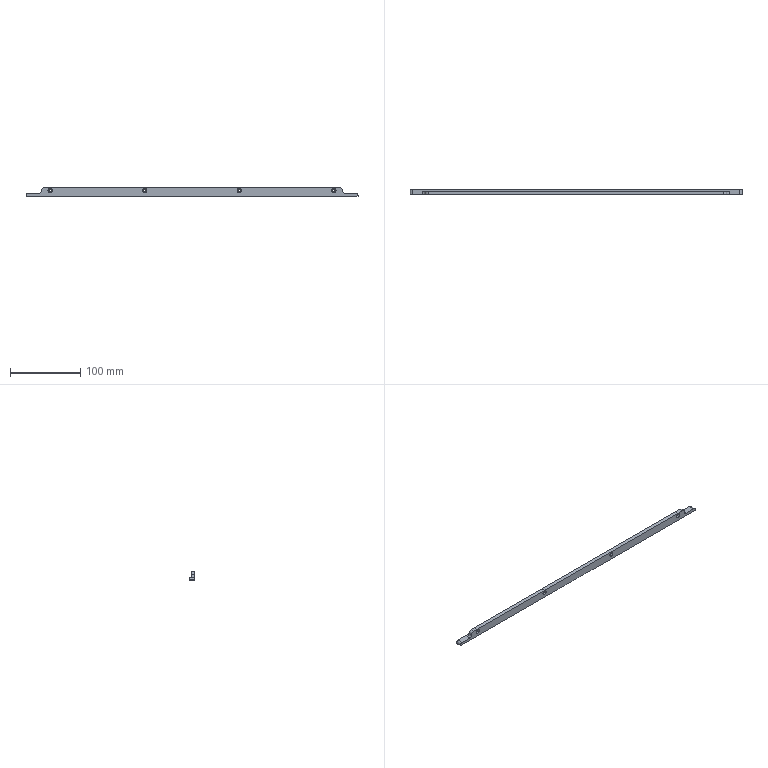Part | NX | 1 solid | 28 faces | box 474 x 8.3 x 12 mm | volume 32389 mm3 | cylinder 14 | plane 14 | commonest cylinder face diameters 3.4 x4 6.5 x4 8 x4 6 x2
STEP:
#1=CARTESIAN_POINT('',(22.,0.,-4.));
#2=VERTEX_POINT('',#1);
#3=CARTESIAN_POINT('',(18.,0.,-8.));
#4=VERTEX_POINT('',#3);
#5=CARTESIAN_POINT('',(18.,0.,-4.));
#6=DIRECTION('',(0.,1.,0.));
#7=DIRECTION('',(0.,0.,-1.));
#8=AXIS2_PLACEMENT_3D('',#5,#6,#7);
#9=CIRCLE('',#8,4.);
#10=EDGE_CURVE('',#2,#4,#9,.T.);
#11=ORIENTED_EDGE('',*,*,#10,.F.);
#12=CARTESIAN_POINT('',(22.,5.,-4.));
#13=VERTEX_POINT('',#12);
#14=CARTESIAN_POINT('',(22.,0.,-4.));
#15=DIRECTION('',(0.,1.,0.));
#16=VECTOR('',#15,1000.);
#17=LINE('',#14,#16);
#18=EDGE_CURVE('',#2,#13,#17,.T.);
#19=ORIENTED_EDGE('',*,*,#18,.T.);
#20=CARTESIAN_POINT('',(18.,5.,-8.));
#21=VERTEX_POINT('',#20);
#22=CARTESIAN_POINT('',(18.,5.,-4.));
#23=DIRECTION('',(0.,-1.,0.));
#24=DIRECTION('',(0.,0.,-1.));
#25=AXIS2_PLACEMENT_3D('',#22,#23,#24);
#26=CIRCLE('',#25,4.);
#27=EDGE_CURVE('',#21,#13,#26,.T.);
#28=ORIENTED_EDGE('',*,*,#27,.F.);
#29=CARTESIAN_POINT('',(18.,8.3,-8.));
#30=DIRECTION('',(0.,1.,0.));
#31=VECTOR('',#30,1000.);
#32=LINE('',#29,#31);
#33=EDGE_CURVE('',#4,#21,#32,.T.);
#34=ORIENTED_EDGE('',*,*,#33,.F.);
#35=EDGE_LOOP('',(#11,#19,#28,#34));
#36=FACE_BOUND('',#35,.T.);
#37=CARTESIAN_POINT('',(18.,-5.,-4.));
#38=DIRECTION('',(0.,1.,0.));
#39=DIRECTION('',(0.,0.,1.));
#40=AXIS2_PLACEMENT_3D('',#37,#38,#39);
#41=CYLINDRICAL_SURFACE('',#40,4.);
#42=ADVANCED_FACE('',(#36),#41,.F.);
#43=ORIENTED_EDGE('',*,*,#18,.F.);
#44=CARTESIAN_POINT('',(26.,0.,0.));
#45=VERTEX_POINT('',#44);
#46=CARTESIAN_POINT('',(26.,0.,-4.));
#47=DIRECTION('',(0.,-1.,0.));
#48=DIRECTION('',(0.,0.,-1.));
#49=AXIS2_PLACEMENT_3D('',#46,#47,#48);
#50=CIRCLE('',#49,4.);
#51=EDGE_CURVE('',#45,#2,#50,.T.);
#52=ORIENTED_EDGE('',*,*,#51,.F.);
#53=CARTESIAN_POINT('',(26.,5.,0.));
#54=VERTEX_POINT('',#53);
#55=CARTESIAN_POINT('',(26.,5.,0.));
#56=DIRECTION('',(0.,1.,0.));
#57=VECTOR('',#56,1000.);
#58=LINE('',#55,#57);
#59=EDGE_CURVE('',#54,#45,#58,.F.);
#60=ORIENTED_EDGE('',*,*,#59,.F.);
#61=CARTESIAN_POINT('',(26.,5.,-4.));
#62=DIRECTION('',(0.,1.,0.));
#63=DIRECTION('',(0.,0.,-1.));
#64=AXIS2_PLACEMENT_3D('',#61,#62,#63);
#65=CIRCLE('',#64,4.);
#66=EDGE_CURVE('',#13,#54,#65,.T.);
#67=ORIENTED_EDGE('',*,*,#66,.F.);
#68=EDGE_LOOP('',(#43,#52,#60,#67));
#69=FACE_BOUND('',#68,.T.);
#70=CARTESIAN_POINT('',(26.,-5.,-4.));
#71=DIRECTION('',(0.,1.,0.));
#72=DIRECTION('',(0.,0.,1.));
#73=AXIS2_PLACEMENT_3D('',#70,#71,#72);
#74=CYLINDRICAL_SURFACE('',#73,4.);
#75=ADVANCED_FACE('',(#69),#74,.T.);
#76=CARTESIAN_POINT('',(452.,0.,-4.));
#77=VERTEX_POINT('',#76);
#78=CARTESIAN_POINT('',(448.,0.,0.));
#79=VERTEX_POINT('',#78);
#80=CARTESIAN_POINT('',(448.,0.,-4.));
#81=DIRECTION('',(0.,-1.,0.));
#82=DIRECTION('',(0.,0.,-1.));
#83=AXIS2_PLACEMENT_3D('',#80,#81,#82);
#84=CIRCLE('',#83,4.);
#85=EDGE_CURVE('',#77,#79,#84,.T.);
#86=ORIENTED_EDGE('',*,*,#85,.F.);
#87=CARTESIAN_POINT('',(452.,5.,-4.));
#88=VERTEX_POINT('',#87);
#89=CARTESIAN_POINT('',(452.,0.,-4.));
#90=DIRECTION('',(0.,-1.,0.));
#91=VECTOR('',#90,1000.);
#92=LINE('',#89,#91);
#93=EDGE_CURVE('',#77,#88,#92,.F.);
#94=ORIENTED_EDGE('',*,*,#93,.T.);
#95=CARTESIAN_POINT('',(448.,5.,0.));
#96=VERTEX_POINT('',#95);
#97=CARTESIAN_POINT('',(448.,5.,-4.));
#98=DIRECTION('',(0.,1.,0.));
#99=DIRECTION('',(0.,0.,-1.));
#100=AXIS2_PLACEMENT_3D('',#97,#98,#99);
#101=CIRCLE('',#100,4.);
#102=EDGE_CURVE('',#96,#88,#101,.T.);
#103=ORIENTED_EDGE('',*,*,#102,.F.);
#104=CARTESIAN_POINT('',(448.,5.,0.));
#105=DIRECTION('',(0.,-1.,0.));
#106=VECTOR('',#105,1000.);
#107=LINE('',#104,#106);
#108=EDGE_CURVE('',#79,#96,#107,.F.);
#109=ORIENTED_EDGE('',*,*,#108,.F.);
#110=EDGE_LOOP('',(#86,#94,#103,#109));
#111=FACE_BOUND('',#110,.T.);
#112=CARTESIAN_POINT('',(448.,-5.,-4.));
#113=DIRECTION('',(0.,-1.,0.));
#114=DIRECTION('',(0.,0.,-1.));
#115=AXIS2_PLACEMENT_3D('',#112,#113,#114);
#116=CYLINDRICAL_SURFACE('',#115,4.);
#117=ADVANCED_FACE('',(#111),#116,.T.);
#118=ORIENTED_EDGE('',*,*,#93,.F.);
#119=CARTESIAN_POINT('',(456.,0.,-8.));
#120=VERTEX_POINT('',#119);
#121=CARTESIAN_POINT('',(456.,0.,-4.));
#122=DIRECTION('',(0.,1.,0.));
#123=DIRECTION('',(0.,0.,-1.));
#124=AXIS2_PLACEMENT_3D('',#121,#122,#123);
#125=CIRCLE('',#124,4.);
#126=EDGE_CURVE('',#120,#77,#125,.T.);
#127=ORIENTED_EDGE('',*,*,#126,.F.);
#128=CARTESIAN_POINT('',(456.,5.,-8.));
#129=VERTEX_POINT('',#128);
#130=CARTESIAN_POINT('',(456.,8.3,-8.));
#131=DIRECTION('',(0.,-1.,0.));
#132=VECTOR('',#131,1000.);
#133=LINE('',#130,#132);
#134=EDGE_CURVE('',#129,#120,#133,.T.);
#135=ORIENTED_EDGE('',*,*,#134,.F.);
#136=CARTESIAN_POINT('',(456.,5.,-4.));
#137=DIRECTION('',(0.,-1.,0.));
#138=DIRECTION('',(0.,0.,-1.));
#139=AXIS2_PLACEMENT_3D('',#136,#137,#138);
#140=CIRCLE('',#139,4.);
#141=EDGE_CURVE('',#88,#129,#140,.T.);
#142=ORIENTED_EDGE('',*,*,#141,.F.);
#143=EDGE_LOOP('',(#118,#127,#135,#142));
#144=FACE_BOUND('',#143,.T.);
#145=CARTESIAN_POINT('',(456.,-5.,-4.));
#146=DIRECTION('',(0.,-1.,0.));
#147=DIRECTION('',(0.,0.,-1.));
#148=AXIS2_PLACEMENT_3D('',#145,#146,#147);
#149=CYLINDRICAL_SURFACE('',#148,4.);
#150=ADVANCED_FACE('',(#144),#149,.F.);
#151=CARTESIAN_POINT('',(34.5,3.4,-7.25));
#152=VERTEX_POINT('',#151);
#153=CARTESIAN_POINT('',(34.5,3.4,-4.));
#154=DIRECTION('',(0.,-1.,0.));
#155=DIRECTION('',(0.,0.,-1.));
#156=AXIS2_PLACEMENT_3D('',#153,#154,#155);
#157=CIRCLE('',#156,3.25);
#158=EDGE_CURVE('',#152,#152,#157,.T.);
#159=ORIENTED_EDGE('',*,*,#158,.T.);
#160=EDGE_LOOP('',(#159));
#161=FACE_BOUND('',#160,.T.);
#162=CARTESIAN_POINT('',(34.5,3.4,-5.7));
#163=VERTEX_POINT('',#162);
#164=CARTESIAN_POINT('',(34.5,3.4,-4.));
#165=DIRECTION('',(0.,-1.,0.));
#166=DIRECTION('',(0.,0.,-1.));
#167=AXIS2_PLACEMENT_3D('',#164,#165,#166);
#168=CIRCLE('',#167,1.7);
#169=EDGE_CURVE('',#163,#163,#168,.T.);
#170=ORIENTED_EDGE('',*,*,#169,.F.);
#171=EDGE_LOOP('',(#170));
#172=FACE_BOUND('',#171,.T.);
#173=CARTESIAN_POINT('',(36.2,3.4,-4.));
#174=DIRECTION('',(0.,1.,0.));
#175=DIRECTION('',(0.,0.,1.));
#176=AXIS2_PLACEMENT_3D('',#173,#174,#175);
#177=PLANE('',#176);
#178=ADVANCED_FACE('',(#161,#172),#177,.F.);
#179=CARTESIAN_POINT('',(169.5,3.4,-0.75));
#180=VERTEX_POINT('',#179);
#181=CARTESIAN_POINT('',(169.5,3.4,-4.));
#182=DIRECTION('',(0.,-1.,0.));
#183=DIRECTION('',(0.,0.,1.));
#184=AXIS2_PLACEMENT_3D('',#181,#182,#183);
#185=CIRCLE('',#184,3.25);
#186=EDGE_CURVE('',#180,#180,#185,.T.);
#187=ORIENTED_EDGE('',*,*,#186,.T.);
#188=EDGE_LOOP('',(#187));
#189=FACE_BOUND('',#188,.T.);
#190=CARTESIAN_POINT('',(169.5,3.4,-2.3));
#191=VERTEX_POINT('',#190);
#192=CARTESIAN_POINT('',(169.5,3.4,-4.));
#193=DIRECTION('',(0.,-1.,0.));
#194=DIRECTION('',(0.,0.,1.));
#195=AXIS2_PLACEMENT_3D('',#192,#193,#194);
#196=CIRCLE('',#195,1.7);
#197=EDGE_CURVE('',#191,#191,#196,.T.);
#198=ORIENTED_EDGE('',*,*,#197,.F.);
#199=EDGE_LOOP('',(#198));
#200=FACE_BOUND('',#199,.T.);
#201=CARTESIAN_POINT('',(36.2,3.4,-4.));
#202=DIRECTION('',(0.,1.,0.));
#203=DIRECTION('',(0.,0.,1.));
#204=AXIS2_PLACEMENT_3D('',#201,#202,#203);
#205=PLANE('',#204);
#206=ADVANCED_FACE('',(#189,#200),#205,.F.);
#207=CARTESIAN_POINT('',(304.5,3.4,-0.75));
#208=VERTEX_POINT('',#207);
#209=CARTESIAN_POINT('',(304.5,3.4,-4.));
#210=DIRECTION('',(0.,-1.,0.));
#211=DIRECTION('',(0.,0.,1.));
#212=AXIS2_PLACEMENT_3D('',#209,#210,#211);
#213=CIRCLE('',#212,3.25);
#214=EDGE_CURVE('',#208,#208,#213,.T.);
#215=ORIENTED_EDGE('',*,*,#214,.T.);
#216=EDGE_LOOP('',(#215));
#217=FACE_BOUND('',#216,.T.);
#218=CARTESIAN_POINT('',(304.5,3.4,-2.3));
#219=VERTEX_POINT('',#218);
#220=CARTESIAN_POINT('',(304.5,3.4,-4.));
#221=DIRECTION('',(0.,-1.,0.));
#222=DIRECTION('',(0.,0.,1.));
#223=AXIS2_PLACEMENT_3D('',#220,#221,#222);
#224=CIRCLE('',#223,1.7);
#225=EDGE_CURVE('',#219,#219,#224,.T.);
#226=ORIENTED_EDGE('',*,*,#225,.F.);
#227=EDGE_LOOP('',(#226));
#228=FACE_BOUND('',#227,.T.);
#229=CARTESIAN_POINT('',(36.2,3.4,-4.));
#230=DIRECTION('',(0.,1.,0.));
#231=DIRECTION('',(0.,0.,1.));
#232=AXIS2_PLACEMENT_3D('',#229,#230,#231);
#233=PLANE('',#232);
#234=ADVANCED_FACE('',(#217,#228),#233,.F.);
#235=CARTESIAN_POINT('',(439.5,3.4,-0.75));
#236=VERTEX_POINT('',#235);
#237=CARTESIAN_POINT('',(439.5,3.4,-4.));
#238=DIRECTION('',(0.,-1.,0.));
#239=DIRECTION('',(0.,0.,1.));
#240=AXIS2_PLACEMENT_3D('',#237,#238,#239);
#241=CIRCLE('',#240,3.25);
#242=EDGE_CURVE('',#236,#236,#241,.T.);
#243=ORIENTED_EDGE('',*,*,#242,.T.);
#244=EDGE_LOOP('',(#243));
#245=FACE_BOUND('',#244,.T.);
#246=CARTESIAN_POINT('',(439.5,3.4,-2.3));
#247=VERTEX_POINT('',#246);
#248=CARTESIAN_POINT('',(439.5,3.4,-4.));
#249=DIRECTION('',(0.,-1.,0.));
#250=DIRECTION('',(0.,0.,1.));
#251=AXIS2_PLACEMENT_3D('',#248,#249,#250);
#252=CIRCLE('',#251,1.7);
#253=EDGE_CURVE('',#247,#247,#252,.T.);
#254=ORIENTED_EDGE('',*,*,#253,.F.);
#255=EDGE_LOOP('',(#254));
#256=FACE_BOUND('',#255,.T.);
#257=CARTESIAN_POINT('',(36.2,3.4,-4.));
#258=DIRECTION('',(0.,1.,0.));
#259=DIRECTION('',(0.,0.,1.));
#260=AXIS2_PLACEMENT_3D('',#257,#258,#259);
#261=PLANE('',#260);
#262=ADVANCED_FACE('',(#245,#256),#261,.F.);
#263=CARTESIAN_POINT('',(471.,8.14,-8.));
#264=VERTEX_POINT('',#263);
#265=CARTESIAN_POINT('',(474.,7.9,-11.));
#266=VERTEX_POINT('',#265);
#267=CARTESIAN_POINT('',(471.,8.14,-11.));
#268=DIRECTION('',(0.07975,0.9968,0.));
#269=DIRECTION('',(0.9968,-0.07975,0.));
#270=AXIS2_PLACEMENT_3D('',#267,#268,#269);
#271=ELLIPSE('',#270,3.01,3.);
#272=EDGE_CURVE('',#264,#266,#271,.T.);
#273=ORIENTED_EDGE('',*,*,#272,.F.);
#274=CARTESIAN_POINT('',(471.,0.,-8.));
#275=VERTEX_POINT('',#274);
#276=CARTESIAN_POINT('',(471.,8.3,-8.));
#277=DIRECTION('',(0.,1.,0.));
#278=VECTOR('',#277,1000.);
#279=LINE('',#276,#278);
#280=EDGE_CURVE('',#275,#264,#279,.T.);
#281=ORIENTED_EDGE('',*,*,#280,.F.);
#282=CARTESIAN_POINT('',(474.,0.,-11.));
#283=VERTEX_POINT('',#282);
#284=CARTESIAN_POINT('',(471.,0.,-11.));
#285=DIRECTION('',(0.,1.,0.));
#286=DIRECTION('',(0.,0.,-1.));
#287=AXIS2_PLACEMENT_3D('',#284,#285,#286);
#288=CIRCLE('',#287,3.);
#289=EDGE_CURVE('',#275,#283,#288,.T.);
#290=ORIENTED_EDGE('',*,*,#289,.T.);
#291=CARTESIAN_POINT('',(474.,5.,-11.));
#292=DIRECTION('',(0.,-1.,0.));
#293=VECTOR('',#292,1000.);
#294=LINE('',#291,#293);
#295=EDGE_CURVE('',#266,#283,#294,.T.);
#296=ORIENTED_EDGE('',*,*,#295,.F.);
#297=EDGE_LOOP('',(#273,#281,#290,#296));
#298=FACE_BOUND('',#297,.T.);
#299=CARTESIAN_POINT('',(471.,5.,-11.));
#300=DIRECTION('',(0.,-1.,0.));
#301=DIRECTION('',(0.,0.,-1.));
#302=AXIS2_PLACEMENT_3D('',#299,#300,#301);
#303=CYLINDRICAL_SURFACE('',#302,3.);
#304=ADVANCED_FACE('',(#298),#303,.T.);
#305=CARTESIAN_POINT('',(0.,7.9,-11.));
#306=VERTEX_POINT('',#305);
#307=CARTESIAN_POINT('',(3.,8.14,-8.));
#308=VERTEX_POINT('',#307);
#309=CARTESIAN_POINT('',(3.,8.14,-11.));
#310=DIRECTION('',(-0.07975,0.9968,0.));
#311=DIRECTION('',(-0.9968,-0.07975,0.));
#312=AXIS2_PLACEMENT_3D('',#309,#310,#311);
#313=ELLIPSE('',#312,3.01,3.);
#314=EDGE_CURVE('',#306,#308,#313,.T.);
#315=ORIENTED_EDGE('',*,*,#314,.F.);
#316=CARTESIAN_POINT('',(0.,0.,-11.));
#317=VERTEX_POINT('',#316);
#318=CARTESIAN_POINT('',(0.,5.,-11.));
#319=DIRECTION('',(0.,1.,0.));
#320=VECTOR('',#319,1000.);
#321=LINE('',#318,#320);
#322=EDGE_CURVE('',#317,#306,#321,.T.);
#323=ORIENTED_EDGE('',*,*,#322,.F.);
#324=CARTESIAN_POINT('',(3.,0.,-8.));
#325=VERTEX_POINT('',#324);
#326=CARTESIAN_POINT('',(3.,0.,-11.));
#327=DIRECTION('',(0.,1.,0.));
#328=DIRECTION('',(0.,0.,-1.));
#329=AXIS2_PLACEMENT_3D('',#326,#327,#328);
#330=CIRCLE('',#329,3.);
#331=EDGE_CURVE('',#317,#325,#330,.T.);
#332=ORIENTED_EDGE('',*,*,#331,.T.);
#333=CARTESIAN_POINT('',(3.,8.3,-8.));
#334=DIRECTION('',(0.,-1.,0.));
#335=VECTOR('',#334,1000.);
#336=LINE('',#333,#335);
#337=EDGE_CURVE('',#308,#325,#336,.T.);
#338=ORIENTED_EDGE('',*,*,#337,.F.);
#339=EDGE_LOOP('',(#315,#323,#332,#338));
#340=FACE_BOUND('',#339,.T.);
#341=CARTESIAN_POINT('',(3.,8.3,-11.));
#342=DIRECTION('',(0.,-1.,0.));
#343=DIRECTION('',(0.,0.,-1.));
#344=AXIS2_PLACEMENT_3D('',#341,#342,#343);
#345=CYLINDRICAL_SURFACE('',#344,3.);
#346=ADVANCED_FACE('',(#340),#345,.T.);
#347=CARTESIAN_POINT('',(469.,8.3,-8.));
#348=VERTEX_POINT('',#347);
#349=CARTESIAN_POINT('',(2.983,45.581,-8.));
#350=DIRECTION('',(-0.9968,0.07975,0.));
#351=VECTOR('',#350,1000.);
#352=LINE('',#349,#351);
#353=EDGE_CURVE('',#264,#348,#352,.T.);
#354=ORIENTED_EDGE('',*,*,#353,.F.);
#355=ORIENTED_EDGE('',*,*,#272,.T.);
#356=CARTESIAN_POINT('',(474.,7.9,-12.));
#357=VERTEX_POINT('',#356);
#358=CARTESIAN_POINT('',(474.,7.9,0.));
#359=DIRECTION('',(0.,0.,-1.));
#360=VECTOR('',#359,1000.);
#361=LINE('',#358,#360);
#362=EDGE_CURVE('',#266,#357,#361,.T.);
#363=ORIENTED_EDGE('',*,*,#362,.T.);
#364=CARTESIAN_POINT('',(469.,8.3,-12.));
#365=VERTEX_POINT('',#364);
#366=CARTESIAN_POINT('',(474.,7.9,-12.));
#367=DIRECTION('',(-0.9968,0.07975,0.));
#368=VECTOR('',#367,1000.);
#369=LINE('',#366,#368);
#370=EDGE_CURVE('',#357,#365,#369,.T.);
#371=ORIENTED_EDGE('',*,*,#370,.T.);
#372=CARTESIAN_POINT('',(469.,8.3,0.));
#373=DIRECTION('',(0.,0.,1.));
#374=VECTOR('',#373,1000.);
#375=LINE('',#372,#374);
#376=EDGE_CURVE('',#365,#348,#375,.T.);
#377=ORIENTED_EDGE('',*,*,#376,.T.);
#378=EDGE_LOOP('',(#354,#355,#363,#371,#377));
#379=FACE_BOUND('',#378,.T.);
#380=CARTESIAN_POINT('',(474.,7.9,0.));
#381=DIRECTION('',(-0.07975,-0.9968,0.));
#382=DIRECTION('',(0.9968,-0.07975,0.));
#383=AXIS2_PLACEMENT_3D('',#380,#381,#382);
#384=PLANE('',#383);
#385=ADVANCED_FACE('',(#379),#384,.F.);
#386=CARTESIAN_POINT('',(0.,7.9,-12.));
#387=VERTEX_POINT('',#386);
#388=CARTESIAN_POINT('',(0.,7.9,0.));
#389=DIRECTION('',(0.,0.,-1.));
#390=VECTOR('',#389,1000.);
#391=LINE('',#388,#390);
#392=EDGE_CURVE('',#306,#387,#391,.T.);
#393=ORIENTED_EDGE('',*,*,#392,.F.);
#394=ORIENTED_EDGE('',*,*,#314,.T.);
#395=CARTESIAN_POINT('',(5.,8.3,-8.));
#396=VERTEX_POINT('',#395);
#397=CARTESIAN_POINT('',(0.0318,7.903,-8.));
#398=DIRECTION('',(-0.9968,-0.07975,0.));
#399=VECTOR('',#398,1000.);
#400=LINE('',#397,#399);
#401=EDGE_CURVE('',#396,#308,#400,.T.);
#402=ORIENTED_EDGE('',*,*,#401,.F.);
#403=CARTESIAN_POINT('',(5.,8.3,-12.));
#404=VERTEX_POINT('',#403);
#405=CARTESIAN_POINT('',(5.,8.3,0.));
#406=DIRECTION('',(0.,0.,-1.));
#407=VECTOR('',#406,1000.);
#408=LINE('',#405,#407);
#409=EDGE_CURVE('',#396,#404,#408,.T.);
#410=ORIENTED_EDGE('',*,*,#409,.T.);
#411=CARTESIAN_POINT('',(5.,8.3,-12.));
#412=DIRECTION('',(-0.9968,-0.07975,0.));
#413=VECTOR('',#412,1000.);
#414=LINE('',#411,#413);
#415=EDGE_CURVE('',#404,#387,#414,.T.);
#416=ORIENTED_EDGE('',*,*,#415,.T.);
#417=EDGE_LOOP('',(#393,#394,#402,#410,#416));
#418=FACE_BOUND('',#417,.T.);
#419=CARTESIAN_POINT('',(5.,8.3,0.));
#420=DIRECTION('',(0.07975,-0.9968,0.));
#421=DIRECTION('',(0.9968,0.07975,0.));
#422=AXIS2_PLACEMENT_3D('',#419,#420,#421);
#423=PLANE('',#422);
#424=ADVANCED_FACE('',(#418),#423,.F.);
#425=ORIENTED_EDGE('',*,*,#376,.F.);
#426=CARTESIAN_POINT('',(0.,8.3,-12.));
#427=DIRECTION('',(-1.,0.,0.));
#428=VECTOR('',#427,1000.);
#429=LINE('',#426,#428);
#430=EDGE_CURVE('',#365,#404,#429,.T.);
#431=ORIENTED_EDGE('',*,*,#430,.T.);
#432=ORIENTED_EDGE('',*,*,#409,.F.);
#433=CARTESIAN_POINT('',(0.,8.3,-8.));
#434=DIRECTION('',(1.,0.,0.));
#435=VECTOR('',#434,1000.);
#436=LINE('',#433,#435);
#437=EDGE_CURVE('',#396,#348,#436,.T.);
#438=ORIENTED_EDGE('',*,*,#437,.T.);
#439=EDGE_LOOP('',(#425,#431,#432,#438));
#440=FACE_BOUND('',#439,.T.);
#441=CARTESIAN_POINT('',(0.,8.3,0.));
#442=DIRECTION('',(0.,1.,0.));
#443=DIRECTION('',(0.,0.,1.));
#444=AXIS2_PLACEMENT_3D('',#441,#442,#443);
#445=PLANE('',#444);
#446=ADVANCED_FACE('',(#440),#445,.T.);
#447=CARTESIAN_POINT('',(0.,5.,-8.));
#448=DIRECTION('',(1.,0.,0.));
#449=VECTOR('',#448,1000.);
#450=LINE('',#447,#449);
#451=EDGE_CURVE('',#21,#129,#450,.T.);
#452=ORIENTED_EDGE('',*,*,#451,.T.);
#453=ORIENTED_EDGE('',*,*,#134,.T.);
#454=CARTESIAN_POINT('',(0.,0.,-8.));
#455=DIRECTION('',(1.,0.,0.));
#456=VECTOR('',#455,1000.);
#457=LINE('',#454,#456);
#458=EDGE_CURVE('',#120,#275,#457,.T.);
#459=ORIENTED_EDGE('',*,*,#458,.T.);
#460=ORIENTED_EDGE('',*,*,#280,.T.);
#461=ORIENTED_EDGE('',*,*,#353,.T.);
#462=ORIENTED_EDGE('',*,*,#437,.F.);
#463=ORIENTED_EDGE('',*,*,#401,.T.);
#464=ORIENTED_EDGE('',*,*,#337,.T.);
#465=CARTESIAN_POINT('',(0.,0.,-8.));
#466=DIRECTION('',(1.,0.,0.));
#467=VECTOR('',#466,1000.);
#468=LINE('',#465,#467);
#469=EDGE_CURVE('',#325,#4,#468,.T.);
#470=ORIENTED_EDGE('',*,*,#469,.T.);
#471=ORIENTED_EDGE('',*,*,#33,.T.);
#472=EDGE_LOOP('',(#452,#453,#459,#460,#461,#462,#463,#464,#470,#471));
#473=FACE_BOUND('',#472,.T.);
#474=CARTESIAN_POINT('',(0.,8.3,-8.));
#475=DIRECTION('',(0.,0.,-1.));
#476=DIRECTION('',(-1.,0.,0.));
#477=AXIS2_PLACEMENT_3D('',#474,#475,#476);
#478=PLANE('',#477);
#479=ADVANCED_FACE('',(#473),#478,.F.);
#480=CARTESIAN_POINT('',(439.5,0.,-7.25));
#481=VERTEX_POINT('',#480);
#482=CARTESIAN_POINT('',(439.5,0.,-4.));
#483=DIRECTION('',(0.,-1.,0.));
#484=DIRECTION('',(0.,0.,-1.));
#485=AXIS2_PLACEMENT_3D('',#482,#483,#484);
#486=CIRCLE('',#485,3.25);
#487=EDGE_CURVE('',#481,#481,#486,.T.);
#488=ORIENTED_EDGE('',*,*,#487,.F.);
#489=EDGE_LOOP('',(#488));
#490=FACE_BOUND('',#489,.T.);
#491=CARTESIAN_POINT('',(304.5,0.,-7.25));
#492=VERTEX_POINT('',#491);
#493=CARTESIAN_POINT('',(304.5,0.,-4.));
#494=DIRECTION('',(0.,-1.,0.));
#495=DIRECTION('',(0.,0.,-1.));
#496=AXIS2_PLACEMENT_3D('',#493,#494,#495);
#497=CIRCLE('',#496,3.25);
#498=EDGE_CURVE('',#492,#492,#497,.T.);
#499=ORIENTED_EDGE('',*,*,#498,.F.);
#500=EDGE_LOOP('',(#499));
#501=FACE_BOUND('',#500,.T.);
#502=CARTESIAN_POINT('',(169.5,0.,-7.25));
#503=VERTEX_POINT('',#502);
#504=CARTESIAN_POINT('',(169.5,0.,-4.));
#505=DIRECTION('',(0.,-1.,0.));
#506=DIRECTION('',(0.,0.,-1.));
#507=AXIS2_PLACEMENT_3D('',#504,#505,#506);
#508=CIRCLE('',#507,3.25);
#509=EDGE_CURVE('',#503,#503,#508,.T.);
#510=ORIENTED_EDGE('',*,*,#509,.F.);
#511=EDGE_LOOP('',(#510));
#512=FACE_BOUND('',#511,.T.);
#513=CARTESIAN_POINT('',(34.5,0.,-7.25));
#514=VERTEX_POINT('',#513);
#515=CARTESIAN_POINT('',(34.5,0.,-4.));
#516=DIRECTION('',(0.,-1.,0.));
#517=DIRECTION('',(0.,0.,-1.));
#518=AXIS2_PLACEMENT_3D('',#515,#516,#517);
#519=CIRCLE('',#518,3.25);
#520=EDGE_CURVE('',#514,#514,#519,.T.);
#521=ORIENTED_EDGE('',*,*,#520,.F.);
#522=EDGE_LOOP('',(#521));
#523=FACE_BOUND('',#522,.T.);
#524=ORIENTED_EDGE('',*,*,#458,.F.);
#525=ORIENTED_EDGE('',*,*,#126,.T.);
#526=ORIENTED_EDGE('',*,*,#85,.T.);
#527=CARTESIAN_POINT('',(0.,0.,0.));
#528=DIRECTION('',(1.,0.,0.));
#529=VECTOR('',#528,1000.);
#530=LINE('',#527,#529);
#531=EDGE_CURVE('',#45,#79,#530,.T.);
#532=ORIENTED_EDGE('',*,*,#531,.F.);
#533=ORIENTED_EDGE('',*,*,#51,.T.);
#534=ORIENTED_EDGE('',*,*,#10,.T.);
#535=ORIENTED_EDGE('',*,*,#469,.F.);
#536=ORIENTED_EDGE('',*,*,#331,.F.);
#537=CARTESIAN_POINT('',(0.,0.,-12.));
#538=VERTEX_POINT('',#537);
#539=CARTESIAN_POINT('',(0.,0.,0.));
#540=DIRECTION('',(0.,0.,1.));
#541=VECTOR('',#540,1000.);
#542=LINE('',#539,#541);
#543=EDGE_CURVE('',#538,#317,#542,.T.);
#544=ORIENTED_EDGE('',*,*,#543,.F.);
#545=CARTESIAN_POINT('',(474.,0.,-12.));
#546=VERTEX_POINT('',#545);
#547=CARTESIAN_POINT('',(0.,0.,-12.));
#548=DIRECTION('',(-1.,0.,0.));
#549=VECTOR('',#548,1000.);
#550=LINE('',#547,#549);
#551=EDGE_CURVE('',#546,#538,#550,.T.);
#552=ORIENTED_EDGE('',*,*,#551,.F.);
#553=CARTESIAN_POINT('',(474.,0.,0.));
#554=DIRECTION('',(0.,0.,-1.));
#555=VECTOR('',#554,1000.);
#556=LINE('',#553,#555);
#557=EDGE_CURVE('',#283,#546,#556,.T.);
#558=ORIENTED_EDGE('',*,*,#557,.F.);
#559=ORIENTED_EDGE('',*,*,#289,.F.);
#560=EDGE_LOOP('',(#524,#525,#526,#532,#533,#534,#535,#536,#544,#552,#558,#559));
#561=FACE_BOUND('',#560,.T.);
#562=CARTESIAN_POINT('',(0.,0.,0.));
#563=DIRECTION('',(0.,-1.,0.));
#564=DIRECTION('',(0.,0.,-1.));
#565=AXIS2_PLACEMENT_3D('',#562,#563,#564);
#566=PLANE('',#565);
#567=ADVANCED_FACE('',(#490,#501,#512,#523,#561),#566,.T.);
#568=ORIENTED_EDGE('',*,*,#430,.F.);
#569=ORIENTED_EDGE('',*,*,#370,.F.);
#570=CARTESIAN_POINT('',(474.,5.,-12.));
#571=DIRECTION('',(0.,-1.,0.));
#572=VECTOR('',#571,1000.);
#573=LINE('',#570,#572);
#574=EDGE_CURVE('',#357,#546,#573,.T.);
#575=ORIENTED_EDGE('',*,*,#574,.T.);
#576=ORIENTED_EDGE('',*,*,#551,.T.);
#577=CARTESIAN_POINT('',(0.,5.,-12.));
#578=DIRECTION('',(0.,-1.,0.));
#579=VECTOR('',#578,1000.);
#580=LINE('',#577,#579);
#581=EDGE_CURVE('',#387,#538,#580,.T.);
#582=ORIENTED_EDGE('',*,*,#581,.F.);
#583=ORIENTED_EDGE('',*,*,#415,.F.);
#584=EDGE_LOOP('',(#568,#569,#575,#576,#582,#583));
#585=FACE_BOUND('',#584,.T.);
#586=CARTESIAN_POINT('',(0.,5.,-12.));
#587=DIRECTION('',(0.,0.,1.));
#588=DIRECTION('',(1.,0.,0.));
#589=AXIS2_PLACEMENT_3D('',#586,#587,#588);
#590=PLANE('',#589);
#591=ADVANCED_FACE('',(#585),#590,.F.);
#592=ORIENTED_EDGE('',*,*,#295,.T.);
#593=ORIENTED_EDGE('',*,*,#557,.T.);
#594=ORIENTED_EDGE('',*,*,#574,.F.);
#595=ORIENTED_EDGE('',*,*,#362,.F.);
#596=EDGE_LOOP('',(#592,#593,#594,#595));
#597=FACE_BOUND('',#596,.T.);
#598=CARTESIAN_POINT('',(474.,5.,0.));
#599=DIRECTION('',(-1.,0.,0.));
#600=DIRECTION('',(0.,0.,1.));
#601=AXIS2_PLACEMENT_3D('',#598,#599,#600);
#602=PLANE('',#601);
#603=ADVANCED_FACE('',(#597),#602,.F.);
#604=ORIENTED_EDGE('',*,*,#531,.T.);
#605=ORIENTED_EDGE('',*,*,#108,.T.);
#606=CARTESIAN_POINT('',(0.,5.,0.));
#607=DIRECTION('',(1.,0.,0.));
#608=VECTOR('',#607,1000.);
#609=LINE('',#606,#608);
#610=EDGE_CURVE('',#54,#96,#609,.T.);
#611=ORIENTED_EDGE('',*,*,#610,.F.);
#612=ORIENTED_EDGE('',*,*,#59,.T.);
#613=EDGE_LOOP('',(#604,#605,#611,#612));
#614=FACE_BOUND('',#613,.T.);
#615=CARTESIAN_POINT('',(0.,5.,0.));
#616=DIRECTION('',(0.,0.,-1.));
#617=DIRECTION('',(-1.,0.,0.));
#618=AXIS2_PLACEMENT_3D('',#615,#616,#617);
#619=PLANE('',#618);
#620=ADVANCED_FACE('',(#614),#619,.F.);
#621=ORIENTED_EDGE('',*,*,#610,.T.);
#622=ORIENTED_EDGE('',*,*,#102,.T.);
#623=ORIENTED_EDGE('',*,*,#141,.T.);
#624=ORIENTED_EDGE('',*,*,#451,.F.);
#625=ORIENTED_EDGE('',*,*,#27,.T.);
#626=ORIENTED_EDGE('',*,*,#66,.T.);
#627=EDGE_LOOP('',(#621,#622,#623,#624,#625,#626));
#628=FACE_BOUND('',#627,.T.);
#629=CARTESIAN_POINT('',(439.5,5.,-5.7));
#630=VERTEX_POINT('',#629);
#631=CARTESIAN_POINT('',(439.5,5.,-4.));
#632=DIRECTION('',(0.,-1.,0.));
#633=DIRECTION('',(0.,0.,-1.));
#634=AXIS2_PLACEMENT_3D('',#631,#632,#633);
#635=CIRCLE('',#634,1.7);
#636=EDGE_CURVE('',#630,#630,#635,.T.);
#637=ORIENTED_EDGE('',*,*,#636,.T.);
#638=EDGE_LOOP('',(#637));
#639=FACE_BOUND('',#638,.T.);
#640=CARTESIAN_POINT('',(304.5,5.,-5.7));
#641=VERTEX_POINT('',#640);
#642=CARTESIAN_POINT('',(304.5,5.,-4.));
#643=DIRECTION('',(0.,-1.,0.));
#644=DIRECTION('',(0.,0.,-1.));
#645=AXIS2_PLACEMENT_3D('',#642,#643,#644);
#646=CIRCLE('',#645,1.7);
#647=EDGE_CURVE('',#641,#641,#646,.T.);
#648=ORIENTED_EDGE('',*,*,#647,.T.);
#649=EDGE_LOOP('',(#648));
#650=FACE_BOUND('',#649,.T.);
#651=CARTESIAN_POINT('',(169.5,5.,-5.7));
#652=VERTEX_POINT('',#651);
#653=CARTESIAN_POINT('',(169.5,5.,-4.));
#654=DIRECTION('',(0.,-1.,0.));
#655=DIRECTION('',(0.,0.,-1.));
#656=AXIS2_PLACEMENT_3D('',#653,#654,#655);
#657=CIRCLE('',#656,1.7);
#658=EDGE_CURVE('',#652,#652,#657,.T.);
#659=ORIENTED_EDGE('',*,*,#658,.T.);
#660=EDGE_LOOP('',(#659));
#661=FACE_BOUND('',#660,.T.);
#662=CARTESIAN_POINT('',(34.5,5.,-5.7));
#663=VERTEX_POINT('',#662);
#664=CARTESIAN_POINT('',(34.5,5.,-4.));
#665=DIRECTION('',(0.,-1.,0.));
#666=DIRECTION('',(0.,0.,-1.));
#667=AXIS2_PLACEMENT_3D('',#664,#665,#666);
#668=CIRCLE('',#667,1.7);
#669=EDGE_CURVE('',#663,#663,#668,.T.);
#670=ORIENTED_EDGE('',*,*,#669,.T.);
#671=EDGE_LOOP('',(#670));
#672=FACE_BOUND('',#671,.T.);
#673=CARTESIAN_POINT('',(0.,5.,0.));
#674=DIRECTION('',(0.,-1.,0.));
#675=DIRECTION('',(0.,0.,-1.));
#676=AXIS2_PLACEMENT_3D('',#673,#674,#675);
#677=PLANE('',#676);
#678=ADVANCED_FACE('',(#628,#639,#650,#661,#672),#677,.F.);
#679=ORIENTED_EDGE('',*,*,#543,.T.);
#680=ORIENTED_EDGE('',*,*,#322,.T.);
#681=ORIENTED_EDGE('',*,*,#392,.T.);
#682=ORIENTED_EDGE('',*,*,#581,.T.);
#683=EDGE_LOOP('',(#679,#680,#681,#682));
#684=FACE_BOUND('',#683,.T.);
#685=CARTESIAN_POINT('',(0.,5.,0.));
#686=DIRECTION('',(1.,0.,0.));
#687=DIRECTION('',(0.,0.,-1.));
#688=AXIS2_PLACEMENT_3D('',#685,#686,#687);
#689=PLANE('',#688);
#690=ADVANCED_FACE('',(#684),#689,.F.);
#691=ORIENTED_EDGE('',*,*,#253,.T.);
#692=EDGE_LOOP('',(#691));
#693=FACE_BOUND('',#692,.T.);
#694=ORIENTED_EDGE('',*,*,#636,.F.);
#695=EDGE_LOOP('',(#694));
#696=FACE_BOUND('',#695,.T.);
#697=CARTESIAN_POINT('',(439.5,0.,-4.));
#698=DIRECTION('',(0.,-1.,0.));
#699=DIRECTION('',(0.,0.,-1.));
#700=AXIS2_PLACEMENT_3D('',#697,#698,#699);
#701=CYLINDRICAL_SURFACE('',#700,1.7);
#702=ADVANCED_FACE('',(#693,#696),#701,.F.);
#703=ORIENTED_EDGE('',*,*,#487,.T.);
#704=EDGE_LOOP('',(#703));
#705=FACE_BOUND('',#704,.T.);
#706=ORIENTED_EDGE('',*,*,#242,.F.);
#707=EDGE_LOOP('',(#706));
#708=FACE_BOUND('',#707,.T.);
#709=CARTESIAN_POINT('',(439.5,0.,-4.));
#710=DIRECTION('',(0.,-1.,0.));
#711=DIRECTION('',(0.,0.,-1.));
#712=AXIS2_PLACEMENT_3D('',#709,#710,#711);
#713=CYLINDRICAL_SURFACE('',#712,3.25);
#714=ADVANCED_FACE('',(#705,#708),#713,.F.);
#715=ORIENTED_EDGE('',*,*,#225,.T.);
#716=EDGE_LOOP('',(#715));
#717=FACE_BOUND('',#716,.T.);
#718=ORIENTED_EDGE('',*,*,#647,.F.);
#719=EDGE_LOOP('',(#718));
#720=FACE_BOUND('',#719,.T.);
#721=CARTESIAN_POINT('',(304.5,0.,-4.));
#722=DIRECTION('',(0.,-1.,0.));
#723=DIRECTION('',(0.,0.,-1.));
#724=AXIS2_PLACEMENT_3D('',#721,#722,#723);
#725=CYLINDRICAL_SURFACE('',#724,1.7);
#726=ADVANCED_FACE('',(#717,#720),#725,.F.);
#727=ORIENTED_EDGE('',*,*,#498,.T.);
#728=EDGE_LOOP('',(#727));
#729=FACE_BOUND('',#728,.T.);
#730=ORIENTED_EDGE('',*,*,#214,.F.);
#731=EDGE_LOOP('',(#730));
#732=FACE_BOUND('',#731,.T.);
#733=CARTESIAN_POINT('',(304.5,0.,-4.));
#734=DIRECTION('',(0.,-1.,0.));
#735=DIRECTION('',(0.,0.,-1.));
#736=AXIS2_PLACEMENT_3D('',#733,#734,#735);
#737=CYLINDRICAL_SURFACE('',#736,3.25);
#738=ADVANCED_FACE('',(#729,#732),#737,.F.);
#739=ORIENTED_EDGE('',*,*,#197,.T.);
#740=EDGE_LOOP('',(#739));
#741=FACE_BOUND('',#740,.T.);
#742=ORIENTED_EDGE('',*,*,#658,.F.);
#743=EDGE_LOOP('',(#742));
#744=FACE_BOUND('',#743,.T.);
#745=CARTESIAN_POINT('',(169.5,0.,-4.));
#746=DIRECTION('',(0.,-1.,0.));
#747=DIRECTION('',(0.,0.,-1.));
#748=AXIS2_PLACEMENT_3D('',#745,#746,#747);
#749=CYLINDRICAL_SURFACE('',#748,1.7);
#750=ADVANCED_FACE('',(#741,#744),#749,.F.);
#751=ORIENTED_EDGE('',*,*,#509,.T.);
#752=EDGE_LOOP('',(#751));
#753=FACE_BOUND('',#752,.T.);
#754=ORIENTED_EDGE('',*,*,#186,.F.);
#755=EDGE_LOOP('',(#754));
#756=FACE_BOUND('',#755,.T.);
#757=CARTESIAN_POINT('',(169.5,0.,-4.));
#758=DIRECTION('',(0.,-1.,0.));
#759=DIRECTION('',(0.,0.,-1.));
#760=AXIS2_PLACEMENT_3D('',#757,#758,#759);
#761=CYLINDRICAL_SURFACE('',#760,3.25);
#762=ADVANCED_FACE('',(#753,#756),#761,.F.);
#763=ORIENTED_EDGE('',*,*,#169,.T.);
#764=EDGE_LOOP('',(#763));
#765=FACE_BOUND('',#764,.T.);
#766=ORIENTED_EDGE('',*,*,#669,.F.);
#767=EDGE_LOOP('',(#766));
#768=FACE_BOUND('',#767,.T.);
#769=CARTESIAN_POINT('',(34.5,0.,-4.));
#770=DIRECTION('',(0.,-1.,0.));
#771=DIRECTION('',(0.,0.,-1.));
#772=AXIS2_PLACEMENT_3D('',#769,#770,#771);
#773=CYLINDRICAL_SURFACE('',#772,1.7);
#774=ADVANCED_FACE('',(#765,#768),#773,.F.);
#775=ORIENTED_EDGE('',*,*,#520,.T.);
#776=EDGE_LOOP('',(#775));
#777=FACE_BOUND('',#776,.T.);
#778=ORIENTED_EDGE('',*,*,#158,.F.);
#779=EDGE_LOOP('',(#778));
#780=FACE_BOUND('',#779,.T.);
#781=CARTESIAN_POINT('',(34.5,0.,-4.));
#782=DIRECTION('',(0.,-1.,0.));
#783=DIRECTION('',(0.,0.,-1.));
#784=AXIS2_PLACEMENT_3D('',#781,#782,#783);
#785=CYLINDRICAL_SURFACE('',#784,3.25);
#786=ADVANCED_FACE('',(#777,#780),#785,.F.);
#787=CLOSED_SHELL('',(#42,#75,#117,#150,#178,#206,#234,#262,#304,#346,#385,#424,#446,#479,#567,#591,#603,#620,#678,#690,#702,#714,#726,#738,#750,#762,#774,#786));
#788=MANIFOLD_SOLID_BREP('',#787);
#789=(LENGTH_UNIT()NAMED_UNIT(*)SI_UNIT(.MILLI.,.METRE.));
#790=UNCERTAINTY_MEASURE_WITH_UNIT(LENGTH_MEASURE(0.00001),#789,'','');
#791=(NAMED_UNIT(*)PLANE_ANGLE_UNIT()SI_UNIT($,.RADIAN.));
#792=(NAMED_UNIT(*)SI_UNIT($,.STERADIAN.)SOLID_ANGLE_UNIT());
#793=(GEOMETRIC_REPRESENTATION_CONTEXT(3)GLOBAL_UNCERTAINTY_ASSIGNED_CONTEXT((#790))GLOBAL_UNIT_ASSIGNED_CONTEXT((#789,#791,#792))REPRESENTATION_CONTEXT('',''));
#794=ADVANCED_BREP_SHAPE_REPRESENTATION('',(#788),#793);